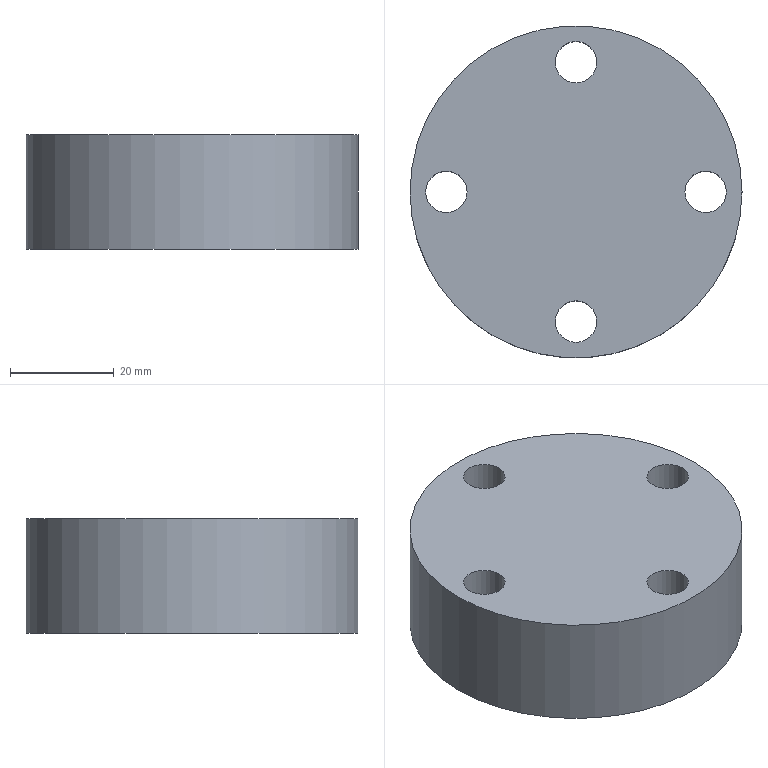CAM job | NX | 3-axis milling, drilling | part box 64 x 64 x 22 mm | stock box 64 x 64 x 22 mm
Tools:
number,name,description,diameter,corner_radius,flute_length,length,flutes
1,ZXZ,Milling Tool-5 Parameters,6.0,0.0,50.0,75.0,2
7,D6A45,Milling Tool-5 Parameters,6.0,0.0,3.0,3.0,2
3,8.0ZT,Drilling Tool,8.0,0.0,35.0,50.0,2
Operations:
program,operation,operation_type,tool,method,geometry_group,spindle_rpm,surface_speed,feed_per_tooth,feed_cut,feed_plunge,cut_length_mm,path_length_mm,cut_time_min,machine_time_min
1,DRILLING,Operation,ZXZ,METHOD,A,3000.0,56.0,0.0333,200.0,0.0,16.0,222.055,0.08,0.1006
1,DRILLING_COPY,Operation,8.0ZT,METHOD,A,1200.0,30.0,0.0625,150.0,0.0,115.614,421.282,0.7708,0.8013
1,ZLEVEL_PROFILE_1_COPY_1,ZLevelMilling,D6A45,METHOD,A,7500.0,141.0,0.0667,1000.0,100.0,105.156,462.767,0.1052,0.1409